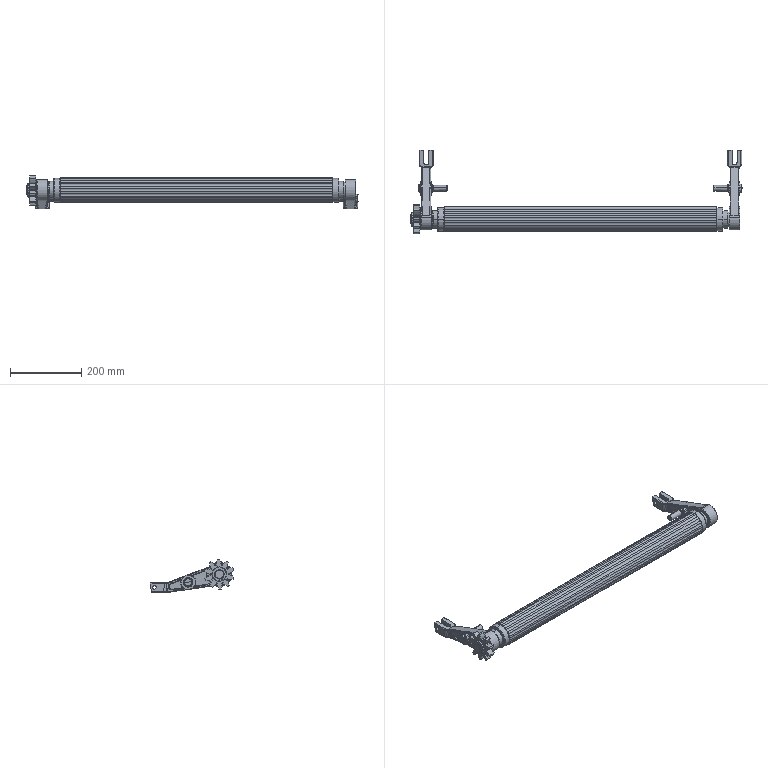Part | SolidWorks | features LayoutProfileFeature 1 | 16 solids | 737 faces | box 934.5 x 236.345 x 93.958 mm | volume 3556008 mm3 | cylinder 313 | spline 206 | plane 132 | cone 86 | commonest cylinder face diameters 4 x72 76.673 x22 14.407 x19 70 x16 25 x15 10 x12